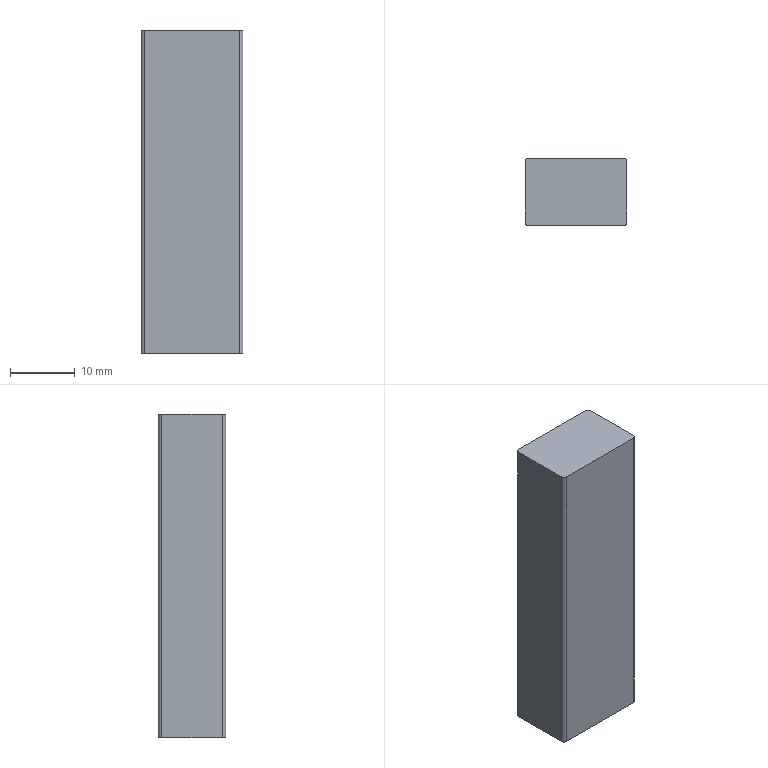Part | NX | features BREP 1 | 1 solid | 10 faces | box 15.7 x 10.4 x 50 mm | volume 8153 mm3 | plane 6 | cylinder 4 | commonest cylinder face diameters 1 x4
STEP:
#1=CARTESIAN_POINT('',(-7.35,5.2,-40.6));
#2=VERTEX_POINT('',#1);
#3=CARTESIAN_POINT('',(-7.85,4.7,-40.6));
#4=VERTEX_POINT('',#3);
#5=CARTESIAN_POINT('',(-7.35,4.7,-40.6));
#6=DIRECTION('',(0.,0.,1.));
#7=DIRECTION('',(1.,0.,0.));
#8=AXIS2_PLACEMENT_3D('',#5,#6,#7);
#9=CIRCLE('',#8,0.5);
#10=EDGE_CURVE('',#2,#4,#9,.T.);
#11=ORIENTED_EDGE('',*,*,#10,.F.);
#12=CARTESIAN_POINT('',(-7.35,5.2,-90.6));
#13=VERTEX_POINT('',#12);
#14=CARTESIAN_POINT('',(-7.35,5.2,-90.6));
#15=DIRECTION('',(0.,0.,1.));
#16=VECTOR('',#15,1000.);
#17=LINE('',#14,#16);
#18=EDGE_CURVE('',#13,#2,#17,.T.);
#19=ORIENTED_EDGE('',*,*,#18,.F.);
#20=CARTESIAN_POINT('',(-7.85,4.7,-90.6));
#21=VERTEX_POINT('',#20);
#22=CARTESIAN_POINT('',(-7.35,4.7,-90.6));
#23=DIRECTION('',(0.,0.,1.));
#24=DIRECTION('',(1.,0.,0.));
#25=AXIS2_PLACEMENT_3D('',#22,#23,#24);
#26=CIRCLE('',#25,0.5);
#27=EDGE_CURVE('',#13,#21,#26,.T.);
#28=ORIENTED_EDGE('',*,*,#27,.T.);
#29=CARTESIAN_POINT('',(-7.85,4.7,-90.6));
#30=DIRECTION('',(0.,0.,1.));
#31=VECTOR('',#30,1000.);
#32=LINE('',#29,#31);
#33=EDGE_CURVE('',#21,#4,#32,.T.);
#34=ORIENTED_EDGE('',*,*,#33,.T.);
#35=EDGE_LOOP('',(#11,#19,#28,#34));
#36=FACE_BOUND('',#35,.T.);
#37=CARTESIAN_POINT('',(-7.35,4.7,-90.6));
#38=DIRECTION('',(0.,0.,1.));
#39=DIRECTION('',(-1.,0.,0.));
#40=AXIS2_PLACEMENT_3D('',#37,#38,#39);
#41=CYLINDRICAL_SURFACE('',#40,0.5);
#42=ADVANCED_FACE('',(#36),#41,.T.);
#43=CARTESIAN_POINT('',(-7.85,-4.7,-40.6));
#44=VERTEX_POINT('',#43);
#45=CARTESIAN_POINT('',(-7.85,-4.7,-40.6));
#46=DIRECTION('',(0.,1.,0.));
#47=VECTOR('',#46,1000.);
#48=LINE('',#45,#47);
#49=EDGE_CURVE('',#44,#4,#48,.T.);
#50=ORIENTED_EDGE('',*,*,#49,.T.);
#51=ORIENTED_EDGE('',*,*,#33,.F.);
#52=CARTESIAN_POINT('',(-7.85,-4.7,-90.6));
#53=VERTEX_POINT('',#52);
#54=CARTESIAN_POINT('',(-7.85,-4.7,-90.6));
#55=DIRECTION('',(0.,1.,0.));
#56=VECTOR('',#55,1000.);
#57=LINE('',#54,#56);
#58=EDGE_CURVE('',#53,#21,#57,.T.);
#59=ORIENTED_EDGE('',*,*,#58,.F.);
#60=CARTESIAN_POINT('',(-7.85,-4.7,-90.6));
#61=DIRECTION('',(0.,0.,1.));
#62=VECTOR('',#61,1000.);
#63=LINE('',#60,#62);
#64=EDGE_CURVE('',#53,#44,#63,.T.);
#65=ORIENTED_EDGE('',*,*,#64,.T.);
#66=EDGE_LOOP('',(#50,#51,#59,#65));
#67=FACE_BOUND('',#66,.T.);
#68=CARTESIAN_POINT('',(-7.85,-4.7,-90.6));
#69=DIRECTION('',(1.,0.,0.));
#70=DIRECTION('',(0.,0.,1.));
#71=AXIS2_PLACEMENT_3D('',#68,#69,#70);
#72=PLANE('',#71);
#73=ADVANCED_FACE('',(#67),#72,.F.);
#74=CARTESIAN_POINT('',(-7.35,-5.2,-40.6));
#75=VERTEX_POINT('',#74);
#76=CARTESIAN_POINT('',(-7.35,-4.7,-40.6));
#77=DIRECTION('',(0.,0.,1.));
#78=DIRECTION('',(1.,0.,0.));
#79=AXIS2_PLACEMENT_3D('',#76,#77,#78);
#80=CIRCLE('',#79,0.5);
#81=EDGE_CURVE('',#44,#75,#80,.T.);
#82=ORIENTED_EDGE('',*,*,#81,.F.);
#83=ORIENTED_EDGE('',*,*,#64,.F.);
#84=CARTESIAN_POINT('',(-7.35,-5.2,-90.6));
#85=VERTEX_POINT('',#84);
#86=CARTESIAN_POINT('',(-7.35,-4.7,-90.6));
#87=DIRECTION('',(0.,0.,1.));
#88=DIRECTION('',(1.,0.,0.));
#89=AXIS2_PLACEMENT_3D('',#86,#87,#88);
#90=CIRCLE('',#89,0.5);
#91=EDGE_CURVE('',#53,#85,#90,.T.);
#92=ORIENTED_EDGE('',*,*,#91,.T.);
#93=CARTESIAN_POINT('',(-7.35,-5.2,-90.6));
#94=DIRECTION('',(0.,0.,1.));
#95=VECTOR('',#94,1000.);
#96=LINE('',#93,#95);
#97=EDGE_CURVE('',#85,#75,#96,.T.);
#98=ORIENTED_EDGE('',*,*,#97,.T.);
#99=EDGE_LOOP('',(#82,#83,#92,#98));
#100=FACE_BOUND('',#99,.T.);
#101=CARTESIAN_POINT('',(-7.35,-4.7,-90.6));
#102=DIRECTION('',(0.,0.,1.));
#103=DIRECTION('',(-1.,0.,0.));
#104=AXIS2_PLACEMENT_3D('',#101,#102,#103);
#105=CYLINDRICAL_SURFACE('',#104,0.5);
#106=ADVANCED_FACE('',(#100),#105,.T.);
#107=CARTESIAN_POINT('',(7.35,-5.2,-40.6));
#108=VERTEX_POINT('',#107);
#109=CARTESIAN_POINT('',(7.35,-5.2,-40.6));
#110=DIRECTION('',(-1.,0.,0.));
#111=VECTOR('',#110,1000.);
#112=LINE('',#109,#111);
#113=EDGE_CURVE('',#108,#75,#112,.T.);
#114=ORIENTED_EDGE('',*,*,#113,.T.);
#115=ORIENTED_EDGE('',*,*,#97,.F.);
#116=CARTESIAN_POINT('',(7.35,-5.2,-90.6));
#117=VERTEX_POINT('',#116);
#118=CARTESIAN_POINT('',(7.35,-5.2,-90.6));
#119=DIRECTION('',(-1.,0.,0.));
#120=VECTOR('',#119,1000.);
#121=LINE('',#118,#120);
#122=EDGE_CURVE('',#117,#85,#121,.T.);
#123=ORIENTED_EDGE('',*,*,#122,.F.);
#124=CARTESIAN_POINT('',(7.35,-5.2,-90.6));
#125=DIRECTION('',(0.,0.,1.));
#126=VECTOR('',#125,1000.);
#127=LINE('',#124,#126);
#128=EDGE_CURVE('',#117,#108,#127,.T.);
#129=ORIENTED_EDGE('',*,*,#128,.T.);
#130=EDGE_LOOP('',(#114,#115,#123,#129));
#131=FACE_BOUND('',#130,.T.);
#132=CARTESIAN_POINT('',(7.35,-5.2,-90.6));
#133=DIRECTION('',(0.,1.,0.));
#134=DIRECTION('',(1.,0.,0.));
#135=AXIS2_PLACEMENT_3D('',#132,#133,#134);
#136=PLANE('',#135);
#137=ADVANCED_FACE('',(#131),#136,.F.);
#138=CARTESIAN_POINT('',(7.85,-4.7,-40.6));
#139=VERTEX_POINT('',#138);
#140=CARTESIAN_POINT('',(7.35,-4.7,-40.6));
#141=DIRECTION('',(0.,0.,1.));
#142=DIRECTION('',(1.,0.,0.));
#143=AXIS2_PLACEMENT_3D('',#140,#141,#142);
#144=CIRCLE('',#143,0.5);
#145=EDGE_CURVE('',#108,#139,#144,.T.);
#146=ORIENTED_EDGE('',*,*,#145,.F.);
#147=ORIENTED_EDGE('',*,*,#128,.F.);
#148=CARTESIAN_POINT('',(7.85,-4.7,-90.6));
#149=VERTEX_POINT('',#148);
#150=CARTESIAN_POINT('',(7.35,-4.7,-90.6));
#151=DIRECTION('',(0.,0.,1.));
#152=DIRECTION('',(1.,0.,0.));
#153=AXIS2_PLACEMENT_3D('',#150,#151,#152);
#154=CIRCLE('',#153,0.5);
#155=EDGE_CURVE('',#117,#149,#154,.T.);
#156=ORIENTED_EDGE('',*,*,#155,.T.);
#157=CARTESIAN_POINT('',(7.85,-4.7,-90.6));
#158=DIRECTION('',(0.,0.,1.));
#159=VECTOR('',#158,1000.);
#160=LINE('',#157,#159);
#161=EDGE_CURVE('',#149,#139,#160,.T.);
#162=ORIENTED_EDGE('',*,*,#161,.T.);
#163=EDGE_LOOP('',(#146,#147,#156,#162));
#164=FACE_BOUND('',#163,.T.);
#165=CARTESIAN_POINT('',(7.35,-4.7,-90.6));
#166=DIRECTION('',(0.,0.,1.));
#167=DIRECTION('',(-1.,0.,0.));
#168=AXIS2_PLACEMENT_3D('',#165,#166,#167);
#169=CYLINDRICAL_SURFACE('',#168,0.5);
#170=ADVANCED_FACE('',(#164),#169,.T.);
#171=CARTESIAN_POINT('',(7.85,4.7,-40.6));
#172=VERTEX_POINT('',#171);
#173=CARTESIAN_POINT('',(7.85,4.7,-40.6));
#174=DIRECTION('',(0.,-1.,0.));
#175=VECTOR('',#174,1000.);
#176=LINE('',#173,#175);
#177=EDGE_CURVE('',#172,#139,#176,.T.);
#178=ORIENTED_EDGE('',*,*,#177,.T.);
#179=ORIENTED_EDGE('',*,*,#161,.F.);
#180=CARTESIAN_POINT('',(7.85,4.7,-90.6));
#181=VERTEX_POINT('',#180);
#182=CARTESIAN_POINT('',(7.85,4.7,-90.6));
#183=DIRECTION('',(0.,-1.,0.));
#184=VECTOR('',#183,1000.);
#185=LINE('',#182,#184);
#186=EDGE_CURVE('',#181,#149,#185,.T.);
#187=ORIENTED_EDGE('',*,*,#186,.F.);
#188=CARTESIAN_POINT('',(7.85,4.7,-90.6));
#189=DIRECTION('',(0.,0.,1.));
#190=VECTOR('',#189,1000.);
#191=LINE('',#188,#190);
#192=EDGE_CURVE('',#181,#172,#191,.T.);
#193=ORIENTED_EDGE('',*,*,#192,.T.);
#194=EDGE_LOOP('',(#178,#179,#187,#193));
#195=FACE_BOUND('',#194,.T.);
#196=CARTESIAN_POINT('',(7.85,4.7,-90.6));
#197=DIRECTION('',(-1.,0.,0.));
#198=DIRECTION('',(0.,1.,0.));
#199=AXIS2_PLACEMENT_3D('',#196,#197,#198);
#200=PLANE('',#199);
#201=ADVANCED_FACE('',(#195),#200,.F.);
#202=CARTESIAN_POINT('',(7.35,5.2,-40.6));
#203=VERTEX_POINT('',#202);
#204=CARTESIAN_POINT('',(7.35,4.7,-40.6));
#205=DIRECTION('',(0.,0.,1.));
#206=DIRECTION('',(1.,0.,0.));
#207=AXIS2_PLACEMENT_3D('',#204,#205,#206);
#208=CIRCLE('',#207,0.5);
#209=EDGE_CURVE('',#172,#203,#208,.T.);
#210=ORIENTED_EDGE('',*,*,#209,.F.);
#211=ORIENTED_EDGE('',*,*,#192,.F.);
#212=CARTESIAN_POINT('',(7.35,5.2,-90.6));
#213=VERTEX_POINT('',#212);
#214=CARTESIAN_POINT('',(7.35,4.7,-90.6));
#215=DIRECTION('',(0.,0.,1.));
#216=DIRECTION('',(1.,0.,0.));
#217=AXIS2_PLACEMENT_3D('',#214,#215,#216);
#218=CIRCLE('',#217,0.5);
#219=EDGE_CURVE('',#181,#213,#218,.T.);
#220=ORIENTED_EDGE('',*,*,#219,.T.);
#221=CARTESIAN_POINT('',(7.35,5.2,-90.6));
#222=DIRECTION('',(0.,0.,1.));
#223=VECTOR('',#222,1000.);
#224=LINE('',#221,#223);
#225=EDGE_CURVE('',#213,#203,#224,.T.);
#226=ORIENTED_EDGE('',*,*,#225,.T.);
#227=EDGE_LOOP('',(#210,#211,#220,#226));
#228=FACE_BOUND('',#227,.T.);
#229=CARTESIAN_POINT('',(7.35,4.7,-90.6));
#230=DIRECTION('',(0.,0.,1.));
#231=DIRECTION('',(-1.,0.,0.));
#232=AXIS2_PLACEMENT_3D('',#229,#230,#231);
#233=CYLINDRICAL_SURFACE('',#232,0.5);
#234=ADVANCED_FACE('',(#228),#233,.T.);
#235=CARTESIAN_POINT('',(-7.35,5.2,-40.6));
#236=DIRECTION('',(1.,0.,0.));
#237=VECTOR('',#236,1000.);
#238=LINE('',#235,#237);
#239=EDGE_CURVE('',#2,#203,#238,.T.);
#240=ORIENTED_EDGE('',*,*,#239,.T.);
#241=ORIENTED_EDGE('',*,*,#225,.F.);
#242=CARTESIAN_POINT('',(-7.35,5.2,-90.6));
#243=DIRECTION('',(1.,0.,0.));
#244=VECTOR('',#243,1000.);
#245=LINE('',#242,#244);
#246=EDGE_CURVE('',#13,#213,#245,.T.);
#247=ORIENTED_EDGE('',*,*,#246,.F.);
#248=ORIENTED_EDGE('',*,*,#18,.T.);
#249=EDGE_LOOP('',(#240,#241,#247,#248));
#250=FACE_BOUND('',#249,.T.);
#251=CARTESIAN_POINT('',(-7.35,5.2,-90.6));
#252=DIRECTION('',(0.,-1.,0.));
#253=DIRECTION('',(0.,0.,1.));
#254=AXIS2_PLACEMENT_3D('',#251,#252,#253);
#255=PLANE('',#254);
#256=ADVANCED_FACE('',(#250),#255,.F.);
#257=ORIENTED_EDGE('',*,*,#27,.F.);
#258=ORIENTED_EDGE('',*,*,#246,.T.);
#259=ORIENTED_EDGE('',*,*,#219,.F.);
#260=ORIENTED_EDGE('',*,*,#186,.T.);
#261=ORIENTED_EDGE('',*,*,#155,.F.);
#262=ORIENTED_EDGE('',*,*,#122,.T.);
#263=ORIENTED_EDGE('',*,*,#91,.F.);
#264=ORIENTED_EDGE('',*,*,#58,.T.);
#265=EDGE_LOOP('',(#257,#258,#259,#260,#261,#262,#263,#264));
#266=FACE_BOUND('',#265,.T.);
#267=CARTESIAN_POINT('',(-7.35,4.7,-90.6));
#268=DIRECTION('',(0.,0.,1.));
#269=DIRECTION('',(-1.,0.,0.));
#270=AXIS2_PLACEMENT_3D('',#267,#268,#269);
#271=PLANE('',#270);
#272=ADVANCED_FACE('',(#266),#271,.F.);
#273=ORIENTED_EDGE('',*,*,#10,.T.);
#274=ORIENTED_EDGE('',*,*,#49,.F.);
#275=ORIENTED_EDGE('',*,*,#81,.T.);
#276=ORIENTED_EDGE('',*,*,#113,.F.);
#277=ORIENTED_EDGE('',*,*,#145,.T.);
#278=ORIENTED_EDGE('',*,*,#177,.F.);
#279=ORIENTED_EDGE('',*,*,#209,.T.);
#280=ORIENTED_EDGE('',*,*,#239,.F.);
#281=EDGE_LOOP('',(#273,#274,#275,#276,#277,#278,#279,#280));
#282=FACE_BOUND('',#281,.T.);
#283=CARTESIAN_POINT('',(-7.35,4.7,-40.6));
#284=DIRECTION('',(0.,0.,1.));
#285=DIRECTION('',(-1.,0.,0.));
#286=AXIS2_PLACEMENT_3D('',#283,#284,#285);
#287=PLANE('',#286);
#288=ADVANCED_FACE('',(#282),#287,.T.);
#289=CLOSED_SHELL('',(#42,#73,#106,#137,#170,#201,#234,#256,#272,#288));
#290=MANIFOLD_SOLID_BREP('',#289);
#291=(LENGTH_UNIT()NAMED_UNIT(*)SI_UNIT(.MILLI.,.METRE.));
#292=UNCERTAINTY_MEASURE_WITH_UNIT(LENGTH_MEASURE(0.00001),#291,'','');
#293=(NAMED_UNIT(*)PLANE_ANGLE_UNIT()SI_UNIT($,.RADIAN.));
#294=(NAMED_UNIT(*)SI_UNIT($,.STERADIAN.)SOLID_ANGLE_UNIT());
#295=(GEOMETRIC_REPRESENTATION_CONTEXT(3)GLOBAL_UNCERTAINTY_ASSIGNED_CONTEXT((#292))GLOBAL_UNIT_ASSIGNED_CONTEXT((#291,#293,#294))REPRESENTATION_CONTEXT('',''));
#296=ADVANCED_BREP_SHAPE_REPRESENTATION('',(#290),#295);